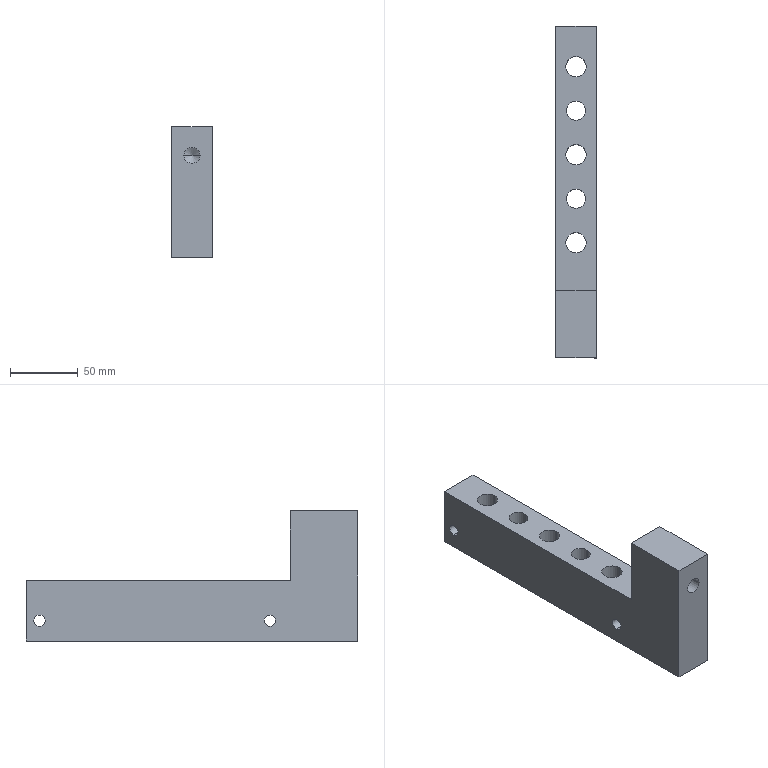Part | STEP file | THANH CHINH NGAM TRUOT 2 | 1 solid | 26 faces | box 30 x 245 x 96 mm | volume 362252 mm3 | cylinder 16 | plane 8 | cone 2 | commonest cylinder face diameters 15 x6 8.376 x4 14 x4 11.835 x2